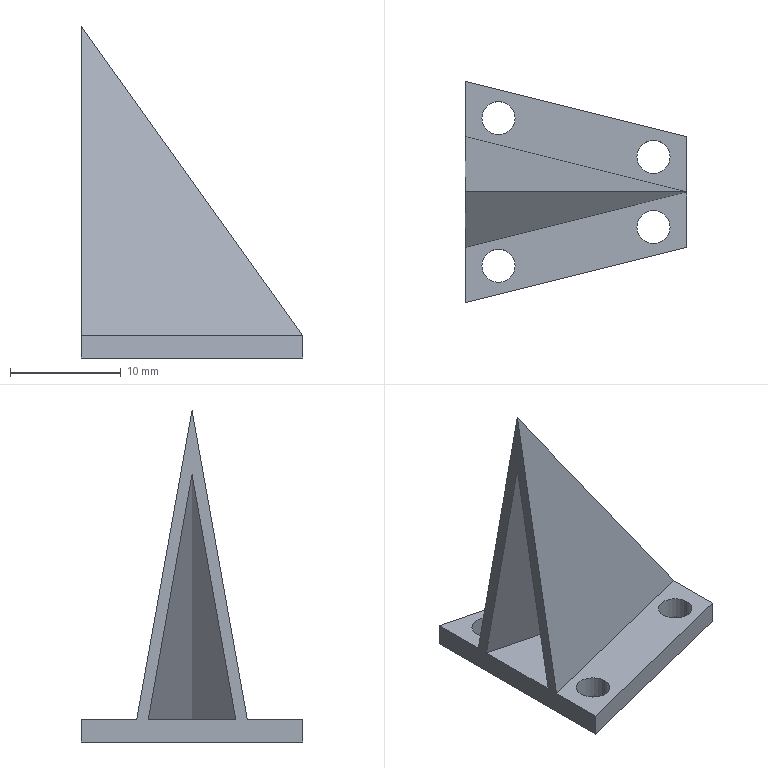Part | SolidWorks | features BaseBody 1 | 1 solid | 20 faces | box 20 x 20 x 30 mm | volume 1015 mm3 | plane 12 | cylinder 8 | commonest cylinder face diameters 3 x8
STEP:
#1=CARTESIAN_POINT('',(1.5,6.673,0.));
#2=VERTEX_POINT('',#1);
#3=CARTESIAN_POINT('',(4.5,6.673,0.));
#4=VERTEX_POINT('',#3);
#5=CARTESIAN_POINT('',(3.,6.673,0.));
#6=DIRECTION('',(0.,0.,-1.));
#7=DIRECTION('',(1.,0.,0.));
#8=AXIS2_PLACEMENT_3D('',#5,#6,#7);
#9=CIRCLE('',#8,1.5);
#10=EDGE_CURVE('',#2,#4,#9,.T.);
#11=ORIENTED_EDGE('',*,*,#10,.F.);
#12=CARTESIAN_POINT('',(1.5,6.673,-2.));
#13=VERTEX_POINT('',#12);
#14=CARTESIAN_POINT('',(1.5,6.673,-2.));
#15=DIRECTION('',(0.,0.,-1.));
#16=VECTOR('',#15,1000.);
#17=LINE('',#14,#16);
#18=EDGE_CURVE('',#2,#13,#17,.T.);
#19=ORIENTED_EDGE('',*,*,#18,.T.);
#20=CARTESIAN_POINT('',(4.5,6.673,-2.));
#21=VERTEX_POINT('',#20);
#22=CARTESIAN_POINT('',(3.,6.673,-2.));
#23=DIRECTION('',(0.,0.,1.));
#24=DIRECTION('',(1.,0.,0.));
#25=AXIS2_PLACEMENT_3D('',#22,#23,#24);
#26=CIRCLE('',#25,1.5);
#27=EDGE_CURVE('',#21,#13,#26,.T.);
#28=ORIENTED_EDGE('',*,*,#27,.F.);
#29=CARTESIAN_POINT('',(4.5,6.673,-2.));
#30=DIRECTION('',(0.,0.,-1.));
#31=VECTOR('',#30,1000.);
#32=LINE('',#29,#31);
#33=EDGE_CURVE('',#4,#21,#32,.T.);
#34=ORIENTED_EDGE('',*,*,#33,.F.);
#35=EDGE_LOOP('',(#11,#19,#28,#34));
#36=FACE_OUTER_BOUND('',#35,.T.);
#37=CARTESIAN_POINT('',(3.,6.673,-2.));
#38=DIRECTION('',(0.,0.,-1.));
#39=DIRECTION('',(1.,0.,0.));
#40=AXIS2_PLACEMENT_3D('',#37,#38,#39);
#41=CYLINDRICAL_SURFACE('',#40,1.5);
#42=ADVANCED_FACE('',(#36),#41,.F.);
#43=CARTESIAN_POINT('',(1.5,-6.673,0.));
#44=VERTEX_POINT('',#43);
#45=CARTESIAN_POINT('',(4.5,-6.673,0.));
#46=VERTEX_POINT('',#45);
#47=CARTESIAN_POINT('',(3.,-6.673,0.));
#48=DIRECTION('',(0.,0.,-1.));
#49=DIRECTION('',(1.,0.,0.));
#50=AXIS2_PLACEMENT_3D('',#47,#48,#49);
#51=CIRCLE('',#50,1.5);
#52=EDGE_CURVE('',#44,#46,#51,.T.);
#53=ORIENTED_EDGE('',*,*,#52,.F.);
#54=CARTESIAN_POINT('',(1.5,-6.673,-2.));
#55=VERTEX_POINT('',#54);
#56=CARTESIAN_POINT('',(1.5,-6.673,-2.));
#57=DIRECTION('',(0.,0.,-1.));
#58=VECTOR('',#57,1000.);
#59=LINE('',#56,#58);
#60=EDGE_CURVE('',#44,#55,#59,.T.);
#61=ORIENTED_EDGE('',*,*,#60,.T.);
#62=CARTESIAN_POINT('',(4.5,-6.673,-2.));
#63=VERTEX_POINT('',#62);
#64=CARTESIAN_POINT('',(3.,-6.673,-2.));
#65=DIRECTION('',(0.,0.,1.));
#66=DIRECTION('',(1.,0.,0.));
#67=AXIS2_PLACEMENT_3D('',#64,#65,#66);
#68=CIRCLE('',#67,1.5);
#69=EDGE_CURVE('',#63,#55,#68,.T.);
#70=ORIENTED_EDGE('',*,*,#69,.F.);
#71=CARTESIAN_POINT('',(4.5,-6.673,-2.));
#72=DIRECTION('',(0.,0.,-1.));
#73=VECTOR('',#72,1000.);
#74=LINE('',#71,#73);
#75=EDGE_CURVE('',#46,#63,#74,.T.);
#76=ORIENTED_EDGE('',*,*,#75,.F.);
#77=EDGE_LOOP('',(#53,#61,#70,#76));
#78=FACE_OUTER_BOUND('',#77,.T.);
#79=CARTESIAN_POINT('',(3.,-6.673,-2.));
#80=DIRECTION('',(0.,0.,-1.));
#81=DIRECTION('',(1.,0.,0.));
#82=AXIS2_PLACEMENT_3D('',#79,#80,#81);
#83=CYLINDRICAL_SURFACE('',#82,1.5);
#84=ADVANCED_FACE('',(#78),#83,.F.);
#85=CARTESIAN_POINT('',(15.5,-3.173,0.));
#86=VERTEX_POINT('',#85);
#87=CARTESIAN_POINT('',(18.5,-3.173,0.));
#88=VERTEX_POINT('',#87);
#89=CARTESIAN_POINT('',(17.,-3.173,0.));
#90=DIRECTION('',(0.,0.,-1.));
#91=DIRECTION('',(1.,0.,0.));
#92=AXIS2_PLACEMENT_3D('',#89,#90,#91);
#93=CIRCLE('',#92,1.5);
#94=EDGE_CURVE('',#86,#88,#93,.T.);
#95=ORIENTED_EDGE('',*,*,#94,.F.);
#96=CARTESIAN_POINT('',(15.5,-3.173,-2.));
#97=VERTEX_POINT('',#96);
#98=CARTESIAN_POINT('',(15.5,-3.173,-2.));
#99=DIRECTION('',(0.,0.,-1.));
#100=VECTOR('',#99,1000.);
#101=LINE('',#98,#100);
#102=EDGE_CURVE('',#86,#97,#101,.T.);
#103=ORIENTED_EDGE('',*,*,#102,.T.);
#104=CARTESIAN_POINT('',(18.5,-3.173,-2.));
#105=VERTEX_POINT('',#104);
#106=CARTESIAN_POINT('',(17.,-3.173,-2.));
#107=DIRECTION('',(0.,0.,1.));
#108=DIRECTION('',(1.,0.,0.));
#109=AXIS2_PLACEMENT_3D('',#106,#107,#108);
#110=CIRCLE('',#109,1.5);
#111=EDGE_CURVE('',#105,#97,#110,.T.);
#112=ORIENTED_EDGE('',*,*,#111,.F.);
#113=CARTESIAN_POINT('',(18.5,-3.173,-2.));
#114=DIRECTION('',(0.,0.,-1.));
#115=VECTOR('',#114,1000.);
#116=LINE('',#113,#115);
#117=EDGE_CURVE('',#88,#105,#116,.T.);
#118=ORIENTED_EDGE('',*,*,#117,.F.);
#119=EDGE_LOOP('',(#95,#103,#112,#118));
#120=FACE_OUTER_BOUND('',#119,.T.);
#121=CARTESIAN_POINT('',(17.,-3.173,-2.));
#122=DIRECTION('',(0.,0.,-1.));
#123=DIRECTION('',(1.,0.,0.));
#124=AXIS2_PLACEMENT_3D('',#121,#122,#123);
#125=CYLINDRICAL_SURFACE('',#124,1.5);
#126=ADVANCED_FACE('',(#120),#125,.F.);
#127=CARTESIAN_POINT('',(15.5,3.173,0.));
#128=VERTEX_POINT('',#127);
#129=CARTESIAN_POINT('',(18.5,3.173,0.));
#130=VERTEX_POINT('',#129);
#131=CARTESIAN_POINT('',(17.,3.173,0.));
#132=DIRECTION('',(0.,0.,-1.));
#133=DIRECTION('',(1.,0.,0.));
#134=AXIS2_PLACEMENT_3D('',#131,#132,#133);
#135=CIRCLE('',#134,1.5);
#136=EDGE_CURVE('',#128,#130,#135,.T.);
#137=ORIENTED_EDGE('',*,*,#136,.F.);
#138=CARTESIAN_POINT('',(15.5,3.173,-2.));
#139=VERTEX_POINT('',#138);
#140=CARTESIAN_POINT('',(15.5,3.173,-2.));
#141=DIRECTION('',(0.,0.,-1.));
#142=VECTOR('',#141,1000.);
#143=LINE('',#140,#142);
#144=EDGE_CURVE('',#128,#139,#143,.T.);
#145=ORIENTED_EDGE('',*,*,#144,.T.);
#146=CARTESIAN_POINT('',(18.5,3.173,-2.));
#147=VERTEX_POINT('',#146);
#148=CARTESIAN_POINT('',(17.,3.173,-2.));
#149=DIRECTION('',(0.,0.,1.));
#150=DIRECTION('',(1.,0.,0.));
#151=AXIS2_PLACEMENT_3D('',#148,#149,#150);
#152=CIRCLE('',#151,1.5);
#153=EDGE_CURVE('',#147,#139,#152,.T.);
#154=ORIENTED_EDGE('',*,*,#153,.F.);
#155=CARTESIAN_POINT('',(18.5,3.173,-2.));
#156=DIRECTION('',(0.,0.,-1.));
#157=VECTOR('',#156,1000.);
#158=LINE('',#155,#157);
#159=EDGE_CURVE('',#130,#147,#158,.T.);
#160=ORIENTED_EDGE('',*,*,#159,.F.);
#161=EDGE_LOOP('',(#137,#145,#154,#160));
#162=FACE_OUTER_BOUND('',#161,.T.);
#163=CARTESIAN_POINT('',(17.,3.173,-2.));
#164=DIRECTION('',(0.,0.,-1.));
#165=DIRECTION('',(1.,0.,0.));
#166=AXIS2_PLACEMENT_3D('',#163,#164,#165);
#167=CYLINDRICAL_SURFACE('',#166,1.5);
#168=ADVANCED_FACE('',(#162),#167,.F.);
#169=CARTESIAN_POINT('',(3.,-6.673,0.));
#170=DIRECTION('',(0.,0.,-1.));
#171=DIRECTION('',(1.,0.,0.));
#172=AXIS2_PLACEMENT_3D('',#169,#170,#171);
#173=CIRCLE('',#172,1.5);
#174=EDGE_CURVE('',#46,#44,#173,.T.);
#175=ORIENTED_EDGE('',*,*,#174,.T.);
#176=ORIENTED_EDGE('',*,*,#52,.T.);
#177=EDGE_LOOP('',(#175,#176));
#178=FACE_BOUND('',#177,.T.);
#179=CARTESIAN_POINT('',(17.,-3.173,0.));
#180=DIRECTION('',(0.,0.,-1.));
#181=DIRECTION('',(1.,0.,0.));
#182=AXIS2_PLACEMENT_3D('',#179,#180,#181);
#183=CIRCLE('',#182,1.5);
#184=EDGE_CURVE('',#88,#86,#183,.T.);
#185=ORIENTED_EDGE('',*,*,#184,.T.);
#186=ORIENTED_EDGE('',*,*,#94,.T.);
#187=EDGE_LOOP('',(#185,#186));
#188=FACE_BOUND('',#187,.T.);
#189=CARTESIAN_POINT('',(20.,0.,0.));
#190=VERTEX_POINT('',#189);
#191=CARTESIAN_POINT('',(0.,-5.,0.));
#192=VERTEX_POINT('',#191);
#193=CARTESIAN_POINT('',(20.,0.,0.));
#194=DIRECTION('',(-0.9701,-0.2425,0.));
#195=VECTOR('',#194,1000.);
#196=LINE('',#193,#195);
#197=EDGE_CURVE('',#190,#192,#196,.T.);
#198=ORIENTED_EDGE('',*,*,#197,.T.);
#199=CARTESIAN_POINT('',(0.,-10.,0.));
#200=VERTEX_POINT('',#199);
#201=CARTESIAN_POINT('',(0.,-10.,0.));
#202=DIRECTION('',(0.,1.,0.));
#203=VECTOR('',#202,1000.);
#204=LINE('',#201,#203);
#205=EDGE_CURVE('',#200,#192,#204,.T.);
#206=ORIENTED_EDGE('',*,*,#205,.F.);
#207=CARTESIAN_POINT('',(20.,-5.,0.));
#208=VERTEX_POINT('',#207);
#209=CARTESIAN_POINT('',(20.,-5.,0.));
#210=DIRECTION('',(-0.9701,-0.2425,0.));
#211=VECTOR('',#210,1000.);
#212=LINE('',#209,#211);
#213=EDGE_CURVE('',#208,#200,#212,.T.);
#214=ORIENTED_EDGE('',*,*,#213,.F.);
#215=CARTESIAN_POINT('',(20.,10.,0.));
#216=DIRECTION('',(0.,-1.,0.));
#217=VECTOR('',#216,1000.);
#218=LINE('',#215,#217);
#219=EDGE_CURVE('',#190,#208,#218,.T.);
#220=ORIENTED_EDGE('',*,*,#219,.F.);
#221=EDGE_LOOP('',(#198,#206,#214,#220));
#222=FACE_OUTER_BOUND('',#221,.T.);
#223=CARTESIAN_POINT('',(8.596,0.,0.));
#224=DIRECTION('',(0.,0.,1.));
#225=DIRECTION('',(1.,0.,0.));
#226=AXIS2_PLACEMENT_3D('',#223,#224,#225);
#227=PLANE('',#226);
#228=ADVANCED_FACE('',(#178,#188,#222),#227,.T.);
#229=CARTESIAN_POINT('',(15.815,0.,0.));
#230=VERTEX_POINT('',#229);
#231=CARTESIAN_POINT('',(0.,3.954,0.));
#232=VERTEX_POINT('',#231);
#233=CARTESIAN_POINT('',(4.129,2.922,0.));
#234=DIRECTION('',(-0.9701,0.2425,0.));
#235=VECTOR('',#234,1000.);
#236=LINE('',#233,#235);
#237=EDGE_CURVE('',#230,#232,#236,.T.);
#238=ORIENTED_EDGE('',*,*,#237,.T.);
#239=CARTESIAN_POINT('',(0.,-3.954,0.));
#240=VERTEX_POINT('',#239);
#241=CARTESIAN_POINT('',(0.,-10.,0.));
#242=DIRECTION('',(0.,1.,0.));
#243=VECTOR('',#242,1000.);
#244=LINE('',#241,#243);
#245=EDGE_CURVE('',#240,#232,#244,.T.);
#246=ORIENTED_EDGE('',*,*,#245,.F.);
#247=CARTESIAN_POINT('',(14.129,-0.4215,0.));
#248=DIRECTION('',(0.9701,0.2425,0.));
#249=VECTOR('',#248,1000.);
#250=LINE('',#247,#249);
#251=EDGE_CURVE('',#240,#230,#250,.T.);
#252=ORIENTED_EDGE('',*,*,#251,.T.);
#253=EDGE_LOOP('',(#238,#246,#252));
#254=FACE_OUTER_BOUND('',#253,.T.);
#255=CARTESIAN_POINT('',(8.596,0.,0.));
#256=DIRECTION('',(0.,0.,1.));
#257=DIRECTION('',(1.,0.,0.));
#258=AXIS2_PLACEMENT_3D('',#255,#256,#257);
#259=PLANE('',#258);
#260=ADVANCED_FACE('',(#254),#259,.T.);
#261=CARTESIAN_POINT('',(3.,6.673,0.));
#262=DIRECTION('',(0.,0.,-1.));
#263=DIRECTION('',(1.,0.,0.));
#264=AXIS2_PLACEMENT_3D('',#261,#262,#263);
#265=CIRCLE('',#264,1.5);
#266=EDGE_CURVE('',#4,#2,#265,.T.);
#267=ORIENTED_EDGE('',*,*,#266,.T.);
#268=ORIENTED_EDGE('',*,*,#10,.T.);
#269=EDGE_LOOP('',(#267,#268));
#270=FACE_BOUND('',#269,.T.);
#271=CARTESIAN_POINT('',(17.,3.173,0.));
#272=DIRECTION('',(0.,0.,-1.));
#273=DIRECTION('',(1.,0.,0.));
#274=AXIS2_PLACEMENT_3D('',#271,#272,#273);
#275=CIRCLE('',#274,1.5);
#276=EDGE_CURVE('',#130,#128,#275,.T.);
#277=ORIENTED_EDGE('',*,*,#276,.T.);
#278=ORIENTED_EDGE('',*,*,#136,.T.);
#279=EDGE_LOOP('',(#277,#278));
#280=FACE_BOUND('',#279,.T.);
#281=CARTESIAN_POINT('',(0.,5.,0.));
#282=VERTEX_POINT('',#281);
#283=CARTESIAN_POINT('',(0.,5.,0.));
#284=DIRECTION('',(0.9701,-0.2425,0.));
#285=VECTOR('',#284,1000.);
#286=LINE('',#283,#285);
#287=EDGE_CURVE('',#282,#190,#286,.T.);
#288=ORIENTED_EDGE('',*,*,#287,.T.);
#289=CARTESIAN_POINT('',(20.,5.,0.));
#290=VERTEX_POINT('',#289);
#291=CARTESIAN_POINT('',(20.,10.,0.));
#292=DIRECTION('',(0.,-1.,0.));
#293=VECTOR('',#292,1000.);
#294=LINE('',#291,#293);
#295=EDGE_CURVE('',#290,#190,#294,.T.);
#296=ORIENTED_EDGE('',*,*,#295,.F.);
#297=CARTESIAN_POINT('',(0.,10.,0.));
#298=VERTEX_POINT('',#297);
#299=CARTESIAN_POINT('',(0.,10.,0.));
#300=DIRECTION('',(0.9701,-0.2425,0.));
#301=VECTOR('',#300,1000.);
#302=LINE('',#299,#301);
#303=EDGE_CURVE('',#298,#290,#302,.T.);
#304=ORIENTED_EDGE('',*,*,#303,.F.);
#305=CARTESIAN_POINT('',(0.,-10.,0.));
#306=DIRECTION('',(0.,1.,0.));
#307=VECTOR('',#306,1000.);
#308=LINE('',#305,#307);
#309=EDGE_CURVE('',#282,#298,#308,.T.);
#310=ORIENTED_EDGE('',*,*,#309,.F.);
#311=EDGE_LOOP('',(#288,#296,#304,#310));
#312=FACE_OUTER_BOUND('',#311,.T.);
#313=CARTESIAN_POINT('',(8.596,0.,0.));
#314=DIRECTION('',(0.,0.,1.));
#315=DIRECTION('',(1.,0.,0.));
#316=AXIS2_PLACEMENT_3D('',#313,#314,#315);
#317=PLANE('',#316);
#318=ADVANCED_FACE('',(#270,#280,#312),#317,.T.);
#319=ORIENTED_EDGE('',*,*,#213,.T.);
#320=CARTESIAN_POINT('',(0.,-10.,-2.));
#321=VERTEX_POINT('',#320);
#322=CARTESIAN_POINT('',(0.,-10.,0.));
#323=DIRECTION('',(0.,0.,-1.));
#324=VECTOR('',#323,1000.);
#325=LINE('',#322,#324);
#326=EDGE_CURVE('',#200,#321,#325,.T.);
#327=ORIENTED_EDGE('',*,*,#326,.T.);
#328=CARTESIAN_POINT('',(20.,-5.,-2.));
#329=VERTEX_POINT('',#328);
#330=CARTESIAN_POINT('',(20.,-5.,-2.));
#331=DIRECTION('',(-0.9701,-0.2425,0.));
#332=VECTOR('',#331,1000.);
#333=LINE('',#330,#332);
#334=EDGE_CURVE('',#329,#321,#333,.T.);
#335=ORIENTED_EDGE('',*,*,#334,.F.);
#336=CARTESIAN_POINT('',(20.,-5.,0.));
#337=DIRECTION('',(0.,0.,-1.));
#338=VECTOR('',#337,1000.);
#339=LINE('',#336,#338);
#340=EDGE_CURVE('',#208,#329,#339,.T.);
#341=ORIENTED_EDGE('',*,*,#340,.F.);
#342=EDGE_LOOP('',(#319,#327,#335,#341));
#343=FACE_OUTER_BOUND('',#342,.T.);
#344=CARTESIAN_POINT('',(20.,-5.,0.));
#345=DIRECTION('',(0.2425,-0.9701,0.));
#346=DIRECTION('',(0.,0.,-1.));
#347=AXIS2_PLACEMENT_3D('',#344,#345,#346);
#348=PLANE('',#347);
#349=ADVANCED_FACE('',(#343),#348,.T.);
#350=ORIENTED_EDGE('',*,*,#295,.T.);
#351=ORIENTED_EDGE('',*,*,#219,.T.);
#352=ORIENTED_EDGE('',*,*,#340,.T.);
#353=CARTESIAN_POINT('',(20.,5.,-2.));
#354=VERTEX_POINT('',#353);
#355=CARTESIAN_POINT('',(20.,10.,-2.));
#356=DIRECTION('',(0.,-1.,0.));
#357=VECTOR('',#356,1000.);
#358=LINE('',#355,#357);
#359=EDGE_CURVE('',#354,#329,#358,.T.);
#360=ORIENTED_EDGE('',*,*,#359,.F.);
#361=CARTESIAN_POINT('',(20.,5.,0.));
#362=DIRECTION('',(0.,0.,-1.));
#363=VECTOR('',#362,1000.);
#364=LINE('',#361,#363);
#365=EDGE_CURVE('',#290,#354,#364,.T.);
#366=ORIENTED_EDGE('',*,*,#365,.F.);
#367=EDGE_LOOP('',(#350,#351,#352,#360,#366));
#368=FACE_OUTER_BOUND('',#367,.T.);
#369=CARTESIAN_POINT('',(20.,5.,0.));
#370=DIRECTION('',(1.,0.,0.));
#371=DIRECTION('',(0.,-1.,0.));
#372=AXIS2_PLACEMENT_3D('',#369,#370,#371);
#373=PLANE('',#372);
#374=ADVANCED_FACE('',(#368),#373,.T.);
#375=ORIENTED_EDGE('',*,*,#303,.T.);
#376=ORIENTED_EDGE('',*,*,#365,.T.);
#377=CARTESIAN_POINT('',(0.,10.,-2.));
#378=VERTEX_POINT('',#377);
#379=CARTESIAN_POINT('',(0.,10.,-2.));
#380=DIRECTION('',(0.9701,-0.2425,0.));
#381=VECTOR('',#380,1000.);
#382=LINE('',#379,#381);
#383=EDGE_CURVE('',#378,#354,#382,.T.);
#384=ORIENTED_EDGE('',*,*,#383,.F.);
#385=CARTESIAN_POINT('',(0.,10.,0.));
#386=DIRECTION('',(0.,0.,-1.));
#387=VECTOR('',#386,1000.);
#388=LINE('',#385,#387);
#389=EDGE_CURVE('',#298,#378,#388,.T.);
#390=ORIENTED_EDGE('',*,*,#389,.F.);
#391=EDGE_LOOP('',(#375,#376,#384,#390));
#392=FACE_OUTER_BOUND('',#391,.T.);
#393=CARTESIAN_POINT('',(0.,10.,0.));
#394=DIRECTION('',(0.2425,0.9701,0.));
#395=DIRECTION('',(0.,0.,-1.));
#396=AXIS2_PLACEMENT_3D('',#393,#394,#395);
#397=PLANE('',#396);
#398=ADVANCED_FACE('',(#392),#397,.T.);
#399=ORIENTED_EDGE('',*,*,#27,.T.);
#400=CARTESIAN_POINT('',(3.,6.673,-2.));
#401=DIRECTION('',(0.,0.,1.));
#402=DIRECTION('',(1.,0.,0.));
#403=AXIS2_PLACEMENT_3D('',#400,#401,#402);
#404=CIRCLE('',#403,1.5);
#405=EDGE_CURVE('',#13,#21,#404,.T.);
#406=ORIENTED_EDGE('',*,*,#405,.T.);
#407=EDGE_LOOP('',(#399,#406));
#408=FACE_BOUND('',#407,.T.);
#409=ORIENTED_EDGE('',*,*,#69,.T.);
#410=CARTESIAN_POINT('',(3.,-6.673,-2.));
#411=DIRECTION('',(0.,0.,1.));
#412=DIRECTION('',(1.,0.,0.));
#413=AXIS2_PLACEMENT_3D('',#410,#411,#412);
#414=CIRCLE('',#413,1.5);
#415=EDGE_CURVE('',#55,#63,#414,.T.);
#416=ORIENTED_EDGE('',*,*,#415,.T.);
#417=EDGE_LOOP('',(#409,#416));
#418=FACE_BOUND('',#417,.T.);
#419=ORIENTED_EDGE('',*,*,#111,.T.);
#420=CARTESIAN_POINT('',(17.,-3.173,-2.));
#421=DIRECTION('',(0.,0.,1.));
#422=DIRECTION('',(1.,0.,0.));
#423=AXIS2_PLACEMENT_3D('',#420,#421,#422);
#424=CIRCLE('',#423,1.5);
#425=EDGE_CURVE('',#97,#105,#424,.T.);
#426=ORIENTED_EDGE('',*,*,#425,.T.);
#427=EDGE_LOOP('',(#419,#426));
#428=FACE_BOUND('',#427,.T.);
#429=ORIENTED_EDGE('',*,*,#153,.T.);
#430=CARTESIAN_POINT('',(17.,3.173,-2.));
#431=DIRECTION('',(0.,0.,1.));
#432=DIRECTION('',(1.,0.,0.));
#433=AXIS2_PLACEMENT_3D('',#430,#431,#432);
#434=CIRCLE('',#433,1.5);
#435=EDGE_CURVE('',#139,#147,#434,.T.);
#436=ORIENTED_EDGE('',*,*,#435,.T.);
#437=EDGE_LOOP('',(#429,#436));
#438=FACE_BOUND('',#437,.T.);
#439=CARTESIAN_POINT('',(0.,-10.,-2.));
#440=DIRECTION('',(0.,1.,0.));
#441=VECTOR('',#440,1000.);
#442=LINE('',#439,#441);
#443=EDGE_CURVE('',#321,#378,#442,.T.);
#444=ORIENTED_EDGE('',*,*,#443,.T.);
#445=ORIENTED_EDGE('',*,*,#383,.T.);
#446=ORIENTED_EDGE('',*,*,#359,.T.);
#447=ORIENTED_EDGE('',*,*,#334,.T.);
#448=EDGE_LOOP('',(#444,#445,#446,#447));
#449=FACE_OUTER_BOUND('',#448,.T.);
#450=CARTESIAN_POINT('',(8.596,0.,-2.));
#451=DIRECTION('',(0.,0.,-1.));
#452=DIRECTION('',(0.,-1.,0.));
#453=AXIS2_PLACEMENT_3D('',#450,#451,#452);
#454=PLANE('',#453);
#455=ADVANCED_FACE('',(#408,#418,#428,#438,#449),#454,.T.);
#456=ORIENTED_EDGE('',*,*,#237,.F.);
#457=CARTESIAN_POINT('',(0.,0.,22.142));
#458=VERTEX_POINT('',#457);
#459=CARTESIAN_POINT('',(13.851,0.,2.751));
#460=DIRECTION('',(-0.5812,0.,0.8137));
#461=VECTOR('',#460,1000.);
#462=LINE('',#459,#461);
#463=EDGE_CURVE('',#230,#458,#462,.T.);
#464=ORIENTED_EDGE('',*,*,#463,.T.);
#465=CARTESIAN_POINT('',(0.,3.832,0.6842));
#466=DIRECTION('',(0.,-0.1758,0.9844));
#467=VECTOR('',#466,1000.);
#468=LINE('',#465,#467);
#469=EDGE_CURVE('',#232,#458,#468,.T.);
#470=ORIENTED_EDGE('',*,*,#469,.F.);
#471=EDGE_LOOP('',(#456,#464,#470));
#472=FACE_OUTER_BOUND('',#471,.T.);
#473=CARTESIAN_POINT('',(-0.239,4.044,-0.1707));
#474=DIRECTION('',(-0.239,-0.9559,-0.1707));
#475=DIRECTION('',(-0.9701,0.2425,0.));
#476=AXIS2_PLACEMENT_3D('',#473,#474,#475);
#477=PLANE('',#476);
#478=ADVANCED_FACE('',(#472),#477,.T.);
#479=ORIENTED_EDGE('',*,*,#251,.F.);
#480=CARTESIAN_POINT('',(0.,-3.909,0.2516));
#481=DIRECTION('',(0.,-0.1758,-0.9844));
#482=VECTOR('',#481,1000.);
#483=LINE('',#480,#482);
#484=EDGE_CURVE('',#458,#240,#483,.T.);
#485=ORIENTED_EDGE('',*,*,#484,.F.);
#486=ORIENTED_EDGE('',*,*,#463,.F.);
#487=EDGE_LOOP('',(#479,#485,#486));
#488=FACE_OUTER_BOUND('',#487,.T.);
#489=CARTESIAN_POINT('',(19.761,0.9559,-0.1707));
#490=DIRECTION('',(-0.239,0.9559,-0.1707));
#491=DIRECTION('',(-0.5812,0.,0.8137));
#492=AXIS2_PLACEMENT_3D('',#489,#490,#491);
#493=PLANE('',#492);
#494=ADVANCED_FACE('',(#488),#493,.T.);
#495=ORIENTED_EDGE('',*,*,#287,.F.);
#496=CARTESIAN_POINT('',(0.,0.,28.));
#497=VERTEX_POINT('',#496);
#498=CARTESIAN_POINT('',(0.,5.,0.));
#499=DIRECTION('',(0.,-0.1758,0.9844));
#500=VECTOR('',#499,1000.);
#501=LINE('',#498,#500);
#502=EDGE_CURVE('',#282,#497,#501,.T.);
#503=ORIENTED_EDGE('',*,*,#502,.T.);
#504=CARTESIAN_POINT('',(20.,0.,0.));
#505=DIRECTION('',(-0.5812,0.,0.8137));
#506=VECTOR('',#505,1000.);
#507=LINE('',#504,#506);
#508=EDGE_CURVE('',#190,#497,#507,.T.);
#509=ORIENTED_EDGE('',*,*,#508,.F.);
#510=EDGE_LOOP('',(#495,#503,#509));
#511=FACE_OUTER_BOUND('',#510,.T.);
#512=CARTESIAN_POINT('',(0.,5.,0.));
#513=DIRECTION('',(-0.239,-0.9559,-0.1707));
#514=DIRECTION('',(-0.9701,0.2425,0.));
#515=AXIS2_PLACEMENT_3D('',#512,#513,#514);
#516=PLANE('',#515);
#517=ADVANCED_FACE('',(#511),#516,.F.);
#518=ORIENTED_EDGE('',*,*,#197,.F.);
#519=ORIENTED_EDGE('',*,*,#508,.T.);
#520=CARTESIAN_POINT('',(0.,-5.,0.));
#521=DIRECTION('',(0.,0.1758,0.9844));
#522=VECTOR('',#521,1000.);
#523=LINE('',#520,#522);
#524=EDGE_CURVE('',#192,#497,#523,.T.);
#525=ORIENTED_EDGE('',*,*,#524,.F.);
#526=EDGE_LOOP('',(#518,#519,#525));
#527=FACE_OUTER_BOUND('',#526,.T.);
#528=CARTESIAN_POINT('',(20.,0.,0.));
#529=DIRECTION('',(-0.239,0.9559,-0.1707));
#530=DIRECTION('',(-0.5812,0.,0.8137));
#531=AXIS2_PLACEMENT_3D('',#528,#529,#530);
#532=PLANE('',#531);
#533=ADVANCED_FACE('',(#527),#532,.F.);
#534=ORIENTED_EDGE('',*,*,#469,.T.);
#535=ORIENTED_EDGE('',*,*,#484,.T.);
#536=ORIENTED_EDGE('',*,*,#245,.T.);
#537=EDGE_LOOP('',(#534,#535,#536));
#538=FACE_BOUND('',#537,.T.);
#539=ORIENTED_EDGE('',*,*,#309,.T.);
#540=ORIENTED_EDGE('',*,*,#389,.T.);
#541=ORIENTED_EDGE('',*,*,#443,.F.);
#542=ORIENTED_EDGE('',*,*,#326,.F.);
#543=ORIENTED_EDGE('',*,*,#205,.T.);
#544=ORIENTED_EDGE('',*,*,#524,.T.);
#545=ORIENTED_EDGE('',*,*,#502,.F.);
#546=EDGE_LOOP('',(#539,#540,#541,#542,#543,#544,#545));
#547=FACE_OUTER_BOUND('',#546,.T.);
#548=CARTESIAN_POINT('',(0.,-5.,0.));
#549=DIRECTION('',(1.,0.,0.));
#550=DIRECTION('',(0.,1.,0.));
#551=AXIS2_PLACEMENT_3D('',#548,#549,#550);
#552=PLANE('',#551);
#553=ADVANCED_FACE('',(#538,#547),#552,.F.);
#554=ORIENTED_EDGE('',*,*,#144,.F.);
#555=ORIENTED_EDGE('',*,*,#276,.F.);
#556=ORIENTED_EDGE('',*,*,#159,.T.);
#557=ORIENTED_EDGE('',*,*,#435,.F.);
#558=EDGE_LOOP('',(#554,#555,#556,#557));
#559=FACE_OUTER_BOUND('',#558,.T.);
#560=CARTESIAN_POINT('',(17.,3.173,-2.));
#561=DIRECTION('',(0.,0.,-1.));
#562=DIRECTION('',(1.,0.,0.));
#563=AXIS2_PLACEMENT_3D('',#560,#561,#562);
#564=CYLINDRICAL_SURFACE('',#563,1.5);
#565=ADVANCED_FACE('',(#559),#564,.F.);
#566=ORIENTED_EDGE('',*,*,#102,.F.);
#567=ORIENTED_EDGE('',*,*,#184,.F.);
#568=ORIENTED_EDGE('',*,*,#117,.T.);
#569=ORIENTED_EDGE('',*,*,#425,.F.);
#570=EDGE_LOOP('',(#566,#567,#568,#569));
#571=FACE_OUTER_BOUND('',#570,.T.);
#572=CARTESIAN_POINT('',(17.,-3.173,-2.));
#573=DIRECTION('',(0.,0.,-1.));
#574=DIRECTION('',(1.,0.,0.));
#575=AXIS2_PLACEMENT_3D('',#572,#573,#574);
#576=CYLINDRICAL_SURFACE('',#575,1.5);
#577=ADVANCED_FACE('',(#571),#576,.F.);
#578=ORIENTED_EDGE('',*,*,#60,.F.);
#579=ORIENTED_EDGE('',*,*,#174,.F.);
#580=ORIENTED_EDGE('',*,*,#75,.T.);
#581=ORIENTED_EDGE('',*,*,#415,.F.);
#582=EDGE_LOOP('',(#578,#579,#580,#581));
#583=FACE_OUTER_BOUND('',#582,.T.);
#584=CARTESIAN_POINT('',(3.,-6.673,-2.));
#585=DIRECTION('',(0.,0.,-1.));
#586=DIRECTION('',(1.,0.,0.));
#587=AXIS2_PLACEMENT_3D('',#584,#585,#586);
#588=CYLINDRICAL_SURFACE('',#587,1.5);
#589=ADVANCED_FACE('',(#583),#588,.F.);
#590=ORIENTED_EDGE('',*,*,#18,.F.);
#591=ORIENTED_EDGE('',*,*,#266,.F.);
#592=ORIENTED_EDGE('',*,*,#33,.T.);
#593=ORIENTED_EDGE('',*,*,#405,.F.);
#594=EDGE_LOOP('',(#590,#591,#592,#593));
#595=FACE_OUTER_BOUND('',#594,.T.);
#596=CARTESIAN_POINT('',(3.,6.673,-2.));
#597=DIRECTION('',(0.,0.,-1.));
#598=DIRECTION('',(1.,0.,0.));
#599=AXIS2_PLACEMENT_3D('',#596,#597,#598);
#600=CYLINDRICAL_SURFACE('',#599,1.5);
#601=ADVANCED_FACE('',(#595),#600,.F.);
#602=CLOSED_SHELL('',(#42,#84,#126,#168,#228,#260,#318,#349,#374,#398,#455,#478,#494,#517,#533,#553,#565,#577,#589,#601));
#603=MANIFOLD_SOLID_BREP('',#602);
#604=CARTESIAN_POINT('',(0.,0.,0.));
#605=DIRECTION('',(0.,0.,1.));
#606=DIRECTION('',(1.,0.,0.));
#607=AXIS2_PLACEMENT_3D('',#604,#605,#606);
#608=(LENGTH_UNIT()NAMED_UNIT(*)SI_UNIT(.MILLI.,.METRE.));
#609=UNCERTAINTY_MEASURE_WITH_UNIT(LENGTH_MEASURE(0.00001),#608,'','');
#610=(NAMED_UNIT(*)PLANE_ANGLE_UNIT()SI_UNIT($,.RADIAN.));
#611=(NAMED_UNIT(*)SI_UNIT($,.STERADIAN.)SOLID_ANGLE_UNIT());
#612=(GEOMETRIC_REPRESENTATION_CONTEXT(3)GLOBAL_UNCERTAINTY_ASSIGNED_CONTEXT((#609))GLOBAL_UNIT_ASSIGNED_CONTEXT((#608,#610,#611))REPRESENTATION_CONTEXT('',''));
#613=ADVANCED_BREP_SHAPE_REPRESENTATION('',(#603,#607),#612);